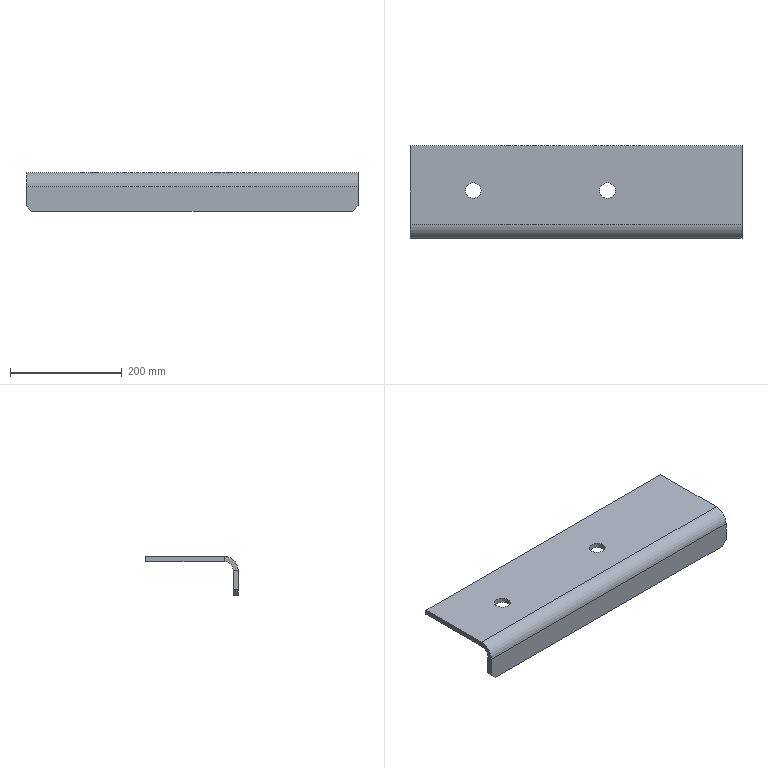Part | SolidWorks | features Chamfer 1, FlatPattern 1, ICE 1, SMBaseFlange 1, SheetMetal 1 | 1 solid | 20 faces | box 593.5 x 165 x 69.5 mm | volume 1145527 mm3 | plane 14 | cylinder 6 | commonest cylinder face diameters 28 x4 32 x1 50 x1
STEP:
#1=CARTESIAN_POINT('',(127.,85.,-9.));
#2=VERTEX_POINT('',#1);
#3=CARTESIAN_POINT('',(99.,85.,-9.));
#4=VERTEX_POINT('',#3);
#5=CARTESIAN_POINT('',(113.,85.,-9.));
#6=DIRECTION('',(0.,0.,-1.));
#7=DIRECTION('',(-1.,0.,0.));
#8=AXIS2_PLACEMENT_3D('',#5,#6,#7);
#9=CIRCLE('',#8,14.);
#10=EDGE_CURVE('',#2,#4,#9,.T.);
#11=ORIENTED_EDGE('',*,*,#10,.T.);
#12=CARTESIAN_POINT('',(99.,85.,0.));
#13=VERTEX_POINT('',#12);
#14=CARTESIAN_POINT('',(99.,85.,-69.5));
#15=DIRECTION('',(0.,0.,1.));
#16=VECTOR('',#15,1000.);
#17=LINE('',#14,#16);
#18=EDGE_CURVE('',#4,#13,#17,.T.);
#19=ORIENTED_EDGE('',*,*,#18,.T.);
#20=CARTESIAN_POINT('',(127.,85.,0.));
#21=VERTEX_POINT('',#20);
#22=CARTESIAN_POINT('',(113.,85.,0.));
#23=DIRECTION('',(0.,0.,1.));
#24=DIRECTION('',(1.,0.,0.));
#25=AXIS2_PLACEMENT_3D('',#22,#23,#24);
#26=CIRCLE('',#25,14.);
#27=EDGE_CURVE('',#13,#21,#26,.T.);
#28=ORIENTED_EDGE('',*,*,#27,.T.);
#29=CARTESIAN_POINT('',(127.,85.,-69.5));
#30=DIRECTION('',(0.,0.,1.));
#31=VECTOR('',#30,1000.);
#32=LINE('',#29,#31);
#33=EDGE_CURVE('',#2,#21,#32,.T.);
#34=ORIENTED_EDGE('',*,*,#33,.F.);
#35=EDGE_LOOP('',(#11,#19,#28,#34));
#36=FACE_OUTER_BOUND('',#35,.T.);
#37=CARTESIAN_POINT('',(113.,85.,-69.5));
#38=DIRECTION('',(0.,0.,1.));
#39=DIRECTION('',(1.,0.,0.));
#40=AXIS2_PLACEMENT_3D('',#37,#38,#39);
#41=CYLINDRICAL_SURFACE('',#40,14.);
#42=ADVANCED_FACE('',(#36),#41,.F.);
#43=CARTESIAN_POINT('',(367.,85.,-9.));
#44=VERTEX_POINT('',#43);
#45=CARTESIAN_POINT('',(339.,85.,-9.));
#46=VERTEX_POINT('',#45);
#47=CARTESIAN_POINT('',(353.,85.,-9.));
#48=DIRECTION('',(0.,0.,-1.));
#49=DIRECTION('',(-1.,0.,0.));
#50=AXIS2_PLACEMENT_3D('',#47,#48,#49);
#51=CIRCLE('',#50,14.);
#52=EDGE_CURVE('',#44,#46,#51,.T.);
#53=ORIENTED_EDGE('',*,*,#52,.T.);
#54=CARTESIAN_POINT('',(339.,85.,0.));
#55=VERTEX_POINT('',#54);
#56=CARTESIAN_POINT('',(339.,85.,-69.5));
#57=DIRECTION('',(0.,0.,1.));
#58=VECTOR('',#57,1000.);
#59=LINE('',#56,#58);
#60=EDGE_CURVE('',#46,#55,#59,.T.);
#61=ORIENTED_EDGE('',*,*,#60,.T.);
#62=CARTESIAN_POINT('',(367.,85.,0.));
#63=VERTEX_POINT('',#62);
#64=CARTESIAN_POINT('',(353.,85.,0.));
#65=DIRECTION('',(0.,0.,1.));
#66=DIRECTION('',(1.,0.,0.));
#67=AXIS2_PLACEMENT_3D('',#64,#65,#66);
#68=CIRCLE('',#67,14.);
#69=EDGE_CURVE('',#55,#63,#68,.T.);
#70=ORIENTED_EDGE('',*,*,#69,.T.);
#71=CARTESIAN_POINT('',(367.,85.,-69.5));
#72=DIRECTION('',(0.,0.,1.));
#73=VECTOR('',#72,1000.);
#74=LINE('',#71,#73);
#75=EDGE_CURVE('',#44,#63,#74,.T.);
#76=ORIENTED_EDGE('',*,*,#75,.F.);
#77=EDGE_LOOP('',(#53,#61,#70,#76));
#78=FACE_OUTER_BOUND('',#77,.T.);
#79=CARTESIAN_POINT('',(353.,85.,-69.5));
#80=DIRECTION('',(0.,0.,1.));
#81=DIRECTION('',(1.,0.,0.));
#82=AXIS2_PLACEMENT_3D('',#79,#80,#81);
#83=CYLINDRICAL_SURFACE('',#82,14.);
#84=ADVANCED_FACE('',(#78),#83,.F.);
#85=CARTESIAN_POINT('',(593.5,25.,0.));
#86=VERTEX_POINT('',#85);
#87=CARTESIAN_POINT('',(593.5,25.,-9.));
#88=VERTEX_POINT('',#87);
#89=CARTESIAN_POINT('',(593.5,25.,0.));
#90=DIRECTION('',(0.,0.,-1.));
#91=VECTOR('',#90,1000.);
#92=LINE('',#89,#91);
#93=EDGE_CURVE('',#86,#88,#92,.T.);
#94=ORIENTED_EDGE('',*,*,#93,.F.);
#95=CARTESIAN_POINT('',(593.5,0.,-25.));
#96=VERTEX_POINT('',#95);
#97=CARTESIAN_POINT('',(593.5,25.,-25.));
#98=DIRECTION('',(1.,0.,0.));
#99=DIRECTION('',(0.,0.,1.));
#100=AXIS2_PLACEMENT_3D('',#97,#98,#99);
#101=CIRCLE('',#100,25.);
#102=EDGE_CURVE('',#86,#96,#101,.T.);
#103=ORIENTED_EDGE('',*,*,#102,.T.);
#104=CARTESIAN_POINT('',(593.5,9.,-25.));
#105=VERTEX_POINT('',#104);
#106=CARTESIAN_POINT('',(593.5,9.,-25.));
#107=DIRECTION('',(0.,-1.,0.));
#108=VECTOR('',#107,1000.);
#109=LINE('',#106,#108);
#110=EDGE_CURVE('',#105,#96,#109,.T.);
#111=ORIENTED_EDGE('',*,*,#110,.F.);
#112=CARTESIAN_POINT('',(593.5,25.,-25.));
#113=DIRECTION('',(1.,0.,0.));
#114=DIRECTION('',(0.,0.,-1.));
#115=AXIS2_PLACEMENT_3D('',#112,#113,#114);
#116=CIRCLE('',#115,16.);
#117=EDGE_CURVE('',#88,#105,#116,.T.);
#118=ORIENTED_EDGE('',*,*,#117,.F.);
#119=EDGE_LOOP('',(#94,#103,#111,#118));
#120=FACE_OUTER_BOUND('',#119,.T.);
#121=CARTESIAN_POINT('',(593.5,25.,0.));
#122=DIRECTION('',(1.,0.,0.));
#123=DIRECTION('',(0.,0.,-1.));
#124=AXIS2_PLACEMENT_3D('',#121,#122,#123);
#125=PLANE('',#124);
#126=ADVANCED_FACE('',(#120),#125,.T.);
#127=CARTESIAN_POINT('',(593.5,165.,0.));
#128=VERTEX_POINT('',#127);
#129=CARTESIAN_POINT('',(593.5,0.,0.));
#130=DIRECTION('',(0.,-1.,0.));
#131=VECTOR('',#130,1000.);
#132=LINE('',#129,#131);
#133=EDGE_CURVE('',#128,#86,#132,.T.);
#134=ORIENTED_EDGE('',*,*,#133,.T.);
#135=ORIENTED_EDGE('',*,*,#93,.T.);
#136=CARTESIAN_POINT('',(593.5,165.,-9.));
#137=VERTEX_POINT('',#136);
#138=CARTESIAN_POINT('',(593.5,0.,-9.));
#139=DIRECTION('',(0.,-1.,0.));
#140=VECTOR('',#139,1000.);
#141=LINE('',#138,#140);
#142=EDGE_CURVE('',#137,#88,#141,.T.);
#143=ORIENTED_EDGE('',*,*,#142,.F.);
#144=CARTESIAN_POINT('',(593.5,165.,0.));
#145=DIRECTION('',(0.,0.,-1.));
#146=VECTOR('',#145,1000.);
#147=LINE('',#144,#146);
#148=EDGE_CURVE('',#128,#137,#147,.T.);
#149=ORIENTED_EDGE('',*,*,#148,.F.);
#150=EDGE_LOOP('',(#134,#135,#143,#149));
#151=FACE_OUTER_BOUND('',#150,.T.);
#152=CARTESIAN_POINT('',(593.5,9.,-25.));
#153=DIRECTION('',(1.,0.,0.));
#154=DIRECTION('',(0.,0.,-1.));
#155=AXIS2_PLACEMENT_3D('',#152,#153,#154);
#156=PLANE('',#155);
#157=ADVANCED_FACE('',(#151),#156,.T.);
#158=CARTESIAN_POINT('',(0.,0.,-25.));
#159=VERTEX_POINT('',#158);
#160=CARTESIAN_POINT('',(0.,9.,-25.));
#161=VERTEX_POINT('',#160);
#162=CARTESIAN_POINT('',(0.,0.,-25.));
#163=DIRECTION('',(0.,1.,0.));
#164=VECTOR('',#163,1000.);
#165=LINE('',#162,#164);
#166=EDGE_CURVE('',#159,#161,#165,.T.);
#167=ORIENTED_EDGE('',*,*,#166,.F.);
#168=CARTESIAN_POINT('',(0.,25.,0.));
#169=VERTEX_POINT('',#168);
#170=CARTESIAN_POINT('',(0.,25.,-25.));
#171=DIRECTION('',(1.,0.,0.));
#172=DIRECTION('',(0.,0.,1.));
#173=AXIS2_PLACEMENT_3D('',#170,#171,#172);
#174=CIRCLE('',#173,25.);
#175=EDGE_CURVE('',#169,#159,#174,.T.);
#176=ORIENTED_EDGE('',*,*,#175,.F.);
#177=CARTESIAN_POINT('',(0.,25.,-9.));
#178=VERTEX_POINT('',#177);
#179=CARTESIAN_POINT('',(0.,25.,-9.));
#180=DIRECTION('',(0.,0.,1.));
#181=VECTOR('',#180,1000.);
#182=LINE('',#179,#181);
#183=EDGE_CURVE('',#178,#169,#182,.T.);
#184=ORIENTED_EDGE('',*,*,#183,.F.);
#185=CARTESIAN_POINT('',(0.,25.,-25.));
#186=DIRECTION('',(1.,0.,0.));
#187=DIRECTION('',(0.,0.,-1.));
#188=AXIS2_PLACEMENT_3D('',#185,#186,#187);
#189=CIRCLE('',#188,16.);
#190=EDGE_CURVE('',#178,#161,#189,.T.);
#191=ORIENTED_EDGE('',*,*,#190,.T.);
#192=EDGE_LOOP('',(#167,#176,#184,#191));
#193=FACE_OUTER_BOUND('',#192,.T.);
#194=CARTESIAN_POINT('',(0.,0.,-25.));
#195=DIRECTION('',(-1.,0.,0.));
#196=DIRECTION('',(0.,0.,1.));
#197=AXIS2_PLACEMENT_3D('',#194,#195,#196);
#198=PLANE('',#197);
#199=ADVANCED_FACE('',(#193),#198,.T.);
#200=CARTESIAN_POINT('',(0.,9.,-59.5));
#201=VERTEX_POINT('',#200);
#202=CARTESIAN_POINT('',(0.,9.,0.));
#203=DIRECTION('',(0.,0.,-1.));
#204=VECTOR('',#203,1000.);
#205=LINE('',#202,#204);
#206=EDGE_CURVE('',#161,#201,#205,.T.);
#207=ORIENTED_EDGE('',*,*,#206,.T.);
#208=CARTESIAN_POINT('',(0.,0.,-59.5));
#209=VERTEX_POINT('',#208);
#210=CARTESIAN_POINT('',(0.,25.,-59.5));
#211=DIRECTION('',(0.,-1.,0.));
#212=VECTOR('',#211,1000.);
#213=LINE('',#210,#212);
#214=EDGE_CURVE('',#201,#209,#213,.T.);
#215=ORIENTED_EDGE('',*,*,#214,.T.);
#216=CARTESIAN_POINT('',(0.,0.,0.));
#217=DIRECTION('',(0.,0.,-1.));
#218=VECTOR('',#217,1000.);
#219=LINE('',#216,#218);
#220=EDGE_CURVE('',#159,#209,#219,.T.);
#221=ORIENTED_EDGE('',*,*,#220,.F.);
#222=ORIENTED_EDGE('',*,*,#166,.T.);
#223=EDGE_LOOP('',(#207,#215,#221,#222));
#224=FACE_OUTER_BOUND('',#223,.T.);
#225=CARTESIAN_POINT('',(0.,25.,-9.));
#226=DIRECTION('',(-1.,0.,0.));
#227=DIRECTION('',(0.,0.,1.));
#228=AXIS2_PLACEMENT_3D('',#225,#226,#227);
#229=PLANE('',#228);
#230=ADVANCED_FACE('',(#224),#229,.T.);
#231=ORIENTED_EDGE('',*,*,#220,.T.);
#232=CARTESIAN_POINT('',(10.,0.,-69.5));
#233=VERTEX_POINT('',#232);
#234=CARTESIAN_POINT('',(0.,0.,-59.5));
#235=DIRECTION('',(0.7071,0.,-0.7071));
#236=VECTOR('',#235,1000.);
#237=LINE('',#234,#236);
#238=EDGE_CURVE('',#209,#233,#237,.T.);
#239=ORIENTED_EDGE('',*,*,#238,.T.);
#240=CARTESIAN_POINT('',(583.5,0.,-69.5));
#241=VERTEX_POINT('',#240);
#242=CARTESIAN_POINT('',(593.5,0.,-69.5));
#243=DIRECTION('',(-1.,0.,0.));
#244=VECTOR('',#243,1000.);
#245=LINE('',#242,#244);
#246=EDGE_CURVE('',#241,#233,#245,.T.);
#247=ORIENTED_EDGE('',*,*,#246,.F.);
#248=CARTESIAN_POINT('',(593.5,0.,-59.5));
#249=VERTEX_POINT('',#248);
#250=CARTESIAN_POINT('',(583.5,0.,-69.5));
#251=DIRECTION('',(0.7071,0.,0.7071));
#252=VECTOR('',#251,1000.);
#253=LINE('',#250,#252);
#254=EDGE_CURVE('',#241,#249,#253,.T.);
#255=ORIENTED_EDGE('',*,*,#254,.T.);
#256=CARTESIAN_POINT('',(593.5,0.,0.));
#257=DIRECTION('',(0.,0.,-1.));
#258=VECTOR('',#257,1000.);
#259=LINE('',#256,#258);
#260=EDGE_CURVE('',#96,#249,#259,.T.);
#261=ORIENTED_EDGE('',*,*,#260,.F.);
#262=CARTESIAN_POINT('',(593.5,0.,-25.));
#263=DIRECTION('',(-1.,0.,0.));
#264=VECTOR('',#263,1000.);
#265=LINE('',#262,#264);
#266=EDGE_CURVE('',#96,#159,#265,.T.);
#267=ORIENTED_EDGE('',*,*,#266,.T.);
#268=EDGE_LOOP('',(#231,#239,#247,#255,#261,#267));
#269=FACE_OUTER_BOUND('',#268,.T.);
#270=CARTESIAN_POINT('',(593.5,0.,0.));
#271=DIRECTION('',(0.,1.,0.));
#272=DIRECTION('',(0.,0.,1.));
#273=AXIS2_PLACEMENT_3D('',#270,#271,#272);
#274=PLANE('',#273);
#275=ADVANCED_FACE('',(#269),#274,.F.);
#276=ORIENTED_EDGE('',*,*,#246,.T.);
#277=CARTESIAN_POINT('',(10.,9.,-69.5));
#278=VERTEX_POINT('',#277);
#279=CARTESIAN_POINT('',(10.,9.,-69.5));
#280=DIRECTION('',(0.,1.,0.));
#281=VECTOR('',#280,1000.);
#282=LINE('',#279,#281);
#283=EDGE_CURVE('',#233,#278,#282,.T.);
#284=ORIENTED_EDGE('',*,*,#283,.T.);
#285=CARTESIAN_POINT('',(583.5,9.,-69.5));
#286=VERTEX_POINT('',#285);
#287=CARTESIAN_POINT('',(593.5,9.,-69.5));
#288=DIRECTION('',(-1.,0.,0.));
#289=VECTOR('',#288,1000.);
#290=LINE('',#287,#289);
#291=EDGE_CURVE('',#286,#278,#290,.T.);
#292=ORIENTED_EDGE('',*,*,#291,.F.);
#293=CARTESIAN_POINT('',(583.5,9.,-69.5));
#294=DIRECTION('',(0.,-1.,0.));
#295=VECTOR('',#294,1000.);
#296=LINE('',#293,#295);
#297=EDGE_CURVE('',#286,#241,#296,.T.);
#298=ORIENTED_EDGE('',*,*,#297,.T.);
#299=EDGE_LOOP('',(#276,#284,#292,#298));
#300=FACE_OUTER_BOUND('',#299,.T.);
#301=CARTESIAN_POINT('',(593.5,9.,-69.5));
#302=DIRECTION('',(0.,0.,-1.));
#303=DIRECTION('',(-1.,0.,0.));
#304=AXIS2_PLACEMENT_3D('',#301,#302,#303);
#305=PLANE('',#304);
#306=ADVANCED_FACE('',(#300),#305,.T.);
#307=ORIENTED_EDGE('',*,*,#291,.T.);
#308=CARTESIAN_POINT('',(267.,9.,-326.5));
#309=DIRECTION('',(-0.7071,0.,0.7071));
#310=VECTOR('',#309,1000.);
#311=LINE('',#308,#310);
#312=EDGE_CURVE('',#278,#201,#311,.T.);
#313=ORIENTED_EDGE('',*,*,#312,.T.);
#314=ORIENTED_EDGE('',*,*,#206,.F.);
#315=CARTESIAN_POINT('',(593.5,9.,-25.));
#316=DIRECTION('',(-1.,0.,0.));
#317=VECTOR('',#316,1000.);
#318=LINE('',#315,#317);
#319=EDGE_CURVE('',#105,#161,#318,.T.);
#320=ORIENTED_EDGE('',*,*,#319,.F.);
#321=CARTESIAN_POINT('',(593.5,9.,-59.5));
#322=VERTEX_POINT('',#321);
#323=CARTESIAN_POINT('',(593.5,9.,0.));
#324=DIRECTION('',(0.,0.,-1.));
#325=VECTOR('',#324,1000.);
#326=LINE('',#323,#325);
#327=EDGE_CURVE('',#105,#322,#326,.T.);
#328=ORIENTED_EDGE('',*,*,#327,.T.);
#329=CARTESIAN_POINT('',(623.25,9.,-29.75));
#330=DIRECTION('',(-0.7071,0.,-0.7071));
#331=VECTOR('',#330,1000.);
#332=LINE('',#329,#331);
#333=EDGE_CURVE('',#322,#286,#332,.T.);
#334=ORIENTED_EDGE('',*,*,#333,.T.);
#335=EDGE_LOOP('',(#307,#313,#314,#320,#328,#334));
#336=FACE_OUTER_BOUND('',#335,.T.);
#337=CARTESIAN_POINT('',(593.5,9.,0.));
#338=DIRECTION('',(0.,1.,0.));
#339=DIRECTION('',(0.,0.,1.));
#340=AXIS2_PLACEMENT_3D('',#337,#338,#339);
#341=PLANE('',#340);
#342=ADVANCED_FACE('',(#336),#341,.T.);
#343=ORIENTED_EDGE('',*,*,#190,.F.);
#344=CARTESIAN_POINT('',(593.5,25.,-9.));
#345=DIRECTION('',(-1.,0.,0.));
#346=VECTOR('',#345,1000.);
#347=LINE('',#344,#346);
#348=EDGE_CURVE('',#88,#178,#347,.T.);
#349=ORIENTED_EDGE('',*,*,#348,.F.);
#350=ORIENTED_EDGE('',*,*,#117,.T.);
#351=ORIENTED_EDGE('',*,*,#319,.T.);
#352=EDGE_LOOP('',(#343,#349,#350,#351));
#353=FACE_OUTER_BOUND('',#352,.T.);
#354=CARTESIAN_POINT('',(593.5,25.,-25.));
#355=DIRECTION('',(-1.,0.,0.));
#356=DIRECTION('',(0.,0.,1.));
#357=AXIS2_PLACEMENT_3D('',#354,#355,#356);
#358=CYLINDRICAL_SURFACE('',#357,16.);
#359=ADVANCED_FACE('',(#353),#358,.F.);
#360=ORIENTED_EDGE('',*,*,#10,.F.);
#361=CARTESIAN_POINT('',(113.,85.,-9.));
#362=DIRECTION('',(0.,0.,-1.));
#363=DIRECTION('',(-1.,0.,0.));
#364=AXIS2_PLACEMENT_3D('',#361,#362,#363);
#365=CIRCLE('',#364,14.);
#366=EDGE_CURVE('',#4,#2,#365,.T.);
#367=ORIENTED_EDGE('',*,*,#366,.F.);
#368=EDGE_LOOP('',(#360,#367));
#369=FACE_BOUND('',#368,.T.);
#370=ORIENTED_EDGE('',*,*,#52,.F.);
#371=CARTESIAN_POINT('',(353.,85.,-9.));
#372=DIRECTION('',(0.,0.,-1.));
#373=DIRECTION('',(-1.,0.,0.));
#374=AXIS2_PLACEMENT_3D('',#371,#372,#373);
#375=CIRCLE('',#374,14.);
#376=EDGE_CURVE('',#46,#44,#375,.T.);
#377=ORIENTED_EDGE('',*,*,#376,.F.);
#378=EDGE_LOOP('',(#370,#377));
#379=FACE_BOUND('',#378,.T.);
#380=CARTESIAN_POINT('',(0.,165.,-9.));
#381=VERTEX_POINT('',#380);
#382=CARTESIAN_POINT('',(0.,0.,-9.));
#383=DIRECTION('',(0.,-1.,0.));
#384=VECTOR('',#383,1000.);
#385=LINE('',#382,#384);
#386=EDGE_CURVE('',#381,#178,#385,.T.);
#387=ORIENTED_EDGE('',*,*,#386,.F.);
#388=CARTESIAN_POINT('',(593.5,165.,-9.));
#389=DIRECTION('',(-1.,0.,0.));
#390=VECTOR('',#389,1000.);
#391=LINE('',#388,#390);
#392=EDGE_CURVE('',#137,#381,#391,.T.);
#393=ORIENTED_EDGE('',*,*,#392,.F.);
#394=ORIENTED_EDGE('',*,*,#142,.T.);
#395=ORIENTED_EDGE('',*,*,#348,.T.);
#396=EDGE_LOOP('',(#387,#393,#394,#395));
#397=FACE_OUTER_BOUND('',#396,.T.);
#398=CARTESIAN_POINT('',(593.5,0.,-9.));
#399=DIRECTION('',(0.,0.,-1.));
#400=DIRECTION('',(-1.,0.,0.));
#401=AXIS2_PLACEMENT_3D('',#398,#399,#400);
#402=PLANE('',#401);
#403=ADVANCED_FACE('',(#369,#379,#397),#402,.T.);
#404=CARTESIAN_POINT('',(0.,165.,0.));
#405=VERTEX_POINT('',#404);
#406=CARTESIAN_POINT('',(0.,165.,0.));
#407=DIRECTION('',(0.,0.,-1.));
#408=VECTOR('',#407,1000.);
#409=LINE('',#406,#408);
#410=EDGE_CURVE('',#405,#381,#409,.T.);
#411=ORIENTED_EDGE('',*,*,#410,.F.);
#412=CARTESIAN_POINT('',(593.5,165.,0.));
#413=DIRECTION('',(-1.,0.,0.));
#414=VECTOR('',#413,1000.);
#415=LINE('',#412,#414);
#416=EDGE_CURVE('',#128,#405,#415,.T.);
#417=ORIENTED_EDGE('',*,*,#416,.F.);
#418=ORIENTED_EDGE('',*,*,#148,.T.);
#419=ORIENTED_EDGE('',*,*,#392,.T.);
#420=EDGE_LOOP('',(#411,#417,#418,#419));
#421=FACE_OUTER_BOUND('',#420,.T.);
#422=CARTESIAN_POINT('',(593.5,165.,0.));
#423=DIRECTION('',(0.,1.,0.));
#424=DIRECTION('',(0.,0.,1.));
#425=AXIS2_PLACEMENT_3D('',#422,#423,#424);
#426=PLANE('',#425);
#427=ADVANCED_FACE('',(#421),#426,.T.);
#428=CARTESIAN_POINT('',(113.,85.,0.));
#429=DIRECTION('',(0.,0.,1.));
#430=DIRECTION('',(1.,0.,0.));
#431=AXIS2_PLACEMENT_3D('',#428,#429,#430);
#432=CIRCLE('',#431,14.);
#433=EDGE_CURVE('',#21,#13,#432,.T.);
#434=ORIENTED_EDGE('',*,*,#433,.F.);
#435=ORIENTED_EDGE('',*,*,#27,.F.);
#436=EDGE_LOOP('',(#434,#435));
#437=FACE_BOUND('',#436,.T.);
#438=CARTESIAN_POINT('',(353.,85.,0.));
#439=DIRECTION('',(0.,0.,1.));
#440=DIRECTION('',(1.,0.,0.));
#441=AXIS2_PLACEMENT_3D('',#438,#439,#440);
#442=CIRCLE('',#441,14.);
#443=EDGE_CURVE('',#63,#55,#442,.T.);
#444=ORIENTED_EDGE('',*,*,#443,.F.);
#445=ORIENTED_EDGE('',*,*,#69,.F.);
#446=EDGE_LOOP('',(#444,#445));
#447=FACE_BOUND('',#446,.T.);
#448=CARTESIAN_POINT('',(0.,0.,0.));
#449=DIRECTION('',(0.,-1.,0.));
#450=VECTOR('',#449,1000.);
#451=LINE('',#448,#450);
#452=EDGE_CURVE('',#405,#169,#451,.T.);
#453=ORIENTED_EDGE('',*,*,#452,.T.);
#454=CARTESIAN_POINT('',(593.5,25.,0.));
#455=DIRECTION('',(-1.,0.,0.));
#456=VECTOR('',#455,1000.);
#457=LINE('',#454,#456);
#458=EDGE_CURVE('',#86,#169,#457,.T.);
#459=ORIENTED_EDGE('',*,*,#458,.F.);
#460=ORIENTED_EDGE('',*,*,#133,.F.);
#461=ORIENTED_EDGE('',*,*,#416,.T.);
#462=EDGE_LOOP('',(#453,#459,#460,#461));
#463=FACE_OUTER_BOUND('',#462,.T.);
#464=CARTESIAN_POINT('',(593.5,0.,0.));
#465=DIRECTION('',(0.,0.,-1.));
#466=DIRECTION('',(-1.,0.,0.));
#467=AXIS2_PLACEMENT_3D('',#464,#465,#466);
#468=PLANE('',#467);
#469=ADVANCED_FACE('',(#437,#447,#463),#468,.F.);
#470=ORIENTED_EDGE('',*,*,#175,.T.);
#471=ORIENTED_EDGE('',*,*,#266,.F.);
#472=ORIENTED_EDGE('',*,*,#102,.F.);
#473=ORIENTED_EDGE('',*,*,#458,.T.);
#474=EDGE_LOOP('',(#470,#471,#472,#473));
#475=FACE_OUTER_BOUND('',#474,.T.);
#476=CARTESIAN_POINT('',(593.5,25.,-25.));
#477=DIRECTION('',(-1.,0.,0.));
#478=DIRECTION('',(0.,0.,1.));
#479=AXIS2_PLACEMENT_3D('',#476,#477,#478);
#480=CYLINDRICAL_SURFACE('',#479,25.);
#481=ADVANCED_FACE('',(#475),#480,.T.);
#482=ORIENTED_EDGE('',*,*,#260,.T.);
#483=CARTESIAN_POINT('',(593.5,25.,-59.5));
#484=DIRECTION('',(0.,1.,0.));
#485=VECTOR('',#484,1000.);
#486=LINE('',#483,#485);
#487=EDGE_CURVE('',#249,#322,#486,.T.);
#488=ORIENTED_EDGE('',*,*,#487,.T.);
#489=ORIENTED_EDGE('',*,*,#327,.F.);
#490=ORIENTED_EDGE('',*,*,#110,.T.);
#491=EDGE_LOOP('',(#482,#488,#489,#490));
#492=FACE_OUTER_BOUND('',#491,.T.);
#493=CARTESIAN_POINT('',(593.5,25.,-25.));
#494=DIRECTION('',(1.,0.,0.));
#495=DIRECTION('',(0.,0.,-1.));
#496=AXIS2_PLACEMENT_3D('',#493,#494,#495);
#497=PLANE('',#496);
#498=ADVANCED_FACE('',(#492),#497,.T.);
#499=ORIENTED_EDGE('',*,*,#386,.T.);
#500=ORIENTED_EDGE('',*,*,#183,.T.);
#501=ORIENTED_EDGE('',*,*,#452,.F.);
#502=ORIENTED_EDGE('',*,*,#410,.T.);
#503=EDGE_LOOP('',(#499,#500,#501,#502));
#504=FACE_OUTER_BOUND('',#503,.T.);
#505=CARTESIAN_POINT('',(0.,25.,-25.));
#506=DIRECTION('',(1.,0.,0.));
#507=DIRECTION('',(0.,0.,-1.));
#508=AXIS2_PLACEMENT_3D('',#505,#506,#507);
#509=PLANE('',#508);
#510=ADVANCED_FACE('',(#504),#509,.F.);
#511=ORIENTED_EDGE('',*,*,#312,.F.);
#512=ORIENTED_EDGE('',*,*,#283,.F.);
#513=ORIENTED_EDGE('',*,*,#238,.F.);
#514=ORIENTED_EDGE('',*,*,#214,.F.);
#515=EDGE_LOOP('',(#511,#512,#513,#514));
#516=FACE_OUTER_BOUND('',#515,.T.);
#517=CARTESIAN_POINT('',(0.,25.,-59.5));
#518=DIRECTION('',(0.7071,0.,0.7071));
#519=DIRECTION('',(0.,-1.,0.));
#520=AXIS2_PLACEMENT_3D('',#517,#518,#519);
#521=PLANE('',#520);
#522=ADVANCED_FACE('',(#516),#521,.F.);
#523=ORIENTED_EDGE('',*,*,#333,.F.);
#524=ORIENTED_EDGE('',*,*,#487,.F.);
#525=ORIENTED_EDGE('',*,*,#254,.F.);
#526=ORIENTED_EDGE('',*,*,#297,.F.);
#527=EDGE_LOOP('',(#523,#524,#525,#526));
#528=FACE_OUTER_BOUND('',#527,.T.);
#529=CARTESIAN_POINT('',(583.5,9.,-69.5));
#530=DIRECTION('',(-0.7071,0.,0.7071));
#531=DIRECTION('',(0.,-1.,0.));
#532=AXIS2_PLACEMENT_3D('',#529,#530,#531);
#533=PLANE('',#532);
#534=ADVANCED_FACE('',(#528),#533,.F.);
#535=ORIENTED_EDGE('',*,*,#60,.F.);
#536=ORIENTED_EDGE('',*,*,#376,.T.);
#537=ORIENTED_EDGE('',*,*,#75,.T.);
#538=ORIENTED_EDGE('',*,*,#443,.T.);
#539=EDGE_LOOP('',(#535,#536,#537,#538));
#540=FACE_OUTER_BOUND('',#539,.T.);
#541=CARTESIAN_POINT('',(353.,85.,-69.5));
#542=DIRECTION('',(0.,0.,1.));
#543=DIRECTION('',(1.,0.,0.));
#544=AXIS2_PLACEMENT_3D('',#541,#542,#543);
#545=CYLINDRICAL_SURFACE('',#544,14.);
#546=ADVANCED_FACE('',(#540),#545,.F.);
#547=ORIENTED_EDGE('',*,*,#18,.F.);
#548=ORIENTED_EDGE('',*,*,#366,.T.);
#549=ORIENTED_EDGE('',*,*,#33,.T.);
#550=ORIENTED_EDGE('',*,*,#433,.T.);
#551=EDGE_LOOP('',(#547,#548,#549,#550));
#552=FACE_OUTER_BOUND('',#551,.T.);
#553=CARTESIAN_POINT('',(113.,85.,-69.5));
#554=DIRECTION('',(0.,0.,1.));
#555=DIRECTION('',(1.,0.,0.));
#556=AXIS2_PLACEMENT_3D('',#553,#554,#555);
#557=CYLINDRICAL_SURFACE('',#556,14.);
#558=ADVANCED_FACE('',(#552),#557,.F.);
#559=CLOSED_SHELL('',(#42,#84,#126,#157,#199,#230,#275,#306,#342,#359,#403,#427,#469,#481,#498,#510,#522,#534,#546,#558));
#560=MANIFOLD_SOLID_BREP('',#559);
#561=CARTESIAN_POINT('',(0.,0.,0.));
#562=DIRECTION('',(0.,0.,1.));
#563=DIRECTION('',(1.,0.,0.));
#564=AXIS2_PLACEMENT_3D('',#561,#562,#563);
#565=(LENGTH_UNIT()NAMED_UNIT(*)SI_UNIT(.MILLI.,.METRE.));
#566=UNCERTAINTY_MEASURE_WITH_UNIT(LENGTH_MEASURE(0.00001),#565,'','');
#567=(NAMED_UNIT(*)PLANE_ANGLE_UNIT()SI_UNIT($,.RADIAN.));
#568=(NAMED_UNIT(*)SI_UNIT($,.STERADIAN.)SOLID_ANGLE_UNIT());
#569=(GEOMETRIC_REPRESENTATION_CONTEXT(3)GLOBAL_UNCERTAINTY_ASSIGNED_CONTEXT((#566))GLOBAL_UNIT_ASSIGNED_CONTEXT((#565,#567,#568))REPRESENTATION_CONTEXT('',''));
#570=ADVANCED_BREP_SHAPE_REPRESENTATION('',(#560,#564),#569);